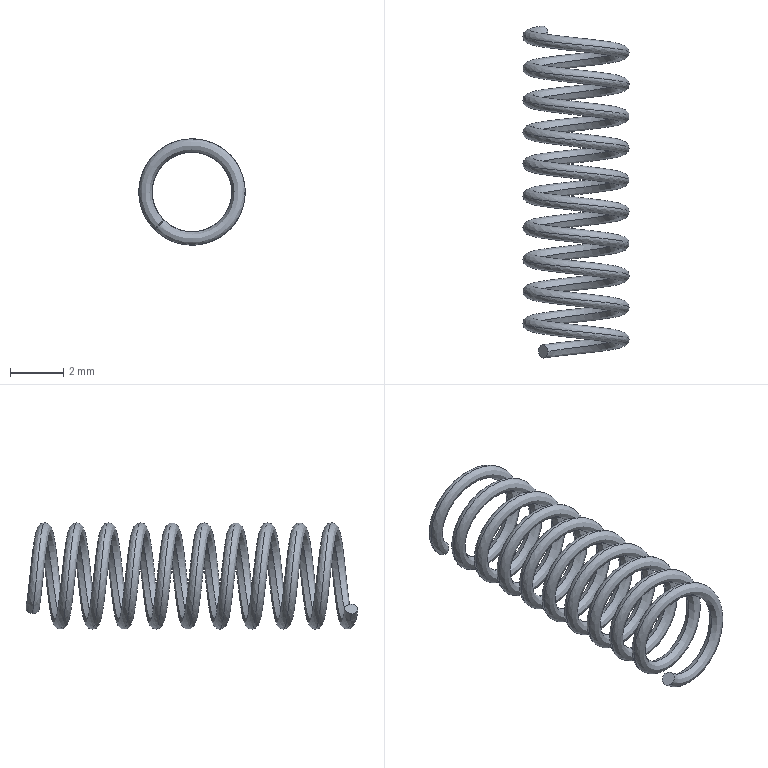Part | NX | features BREP 1 | 1 solid | 4 faces | box 4 x 12.497 x 4 mm | volume 21.567 mm3 | spline 2 | plane 2